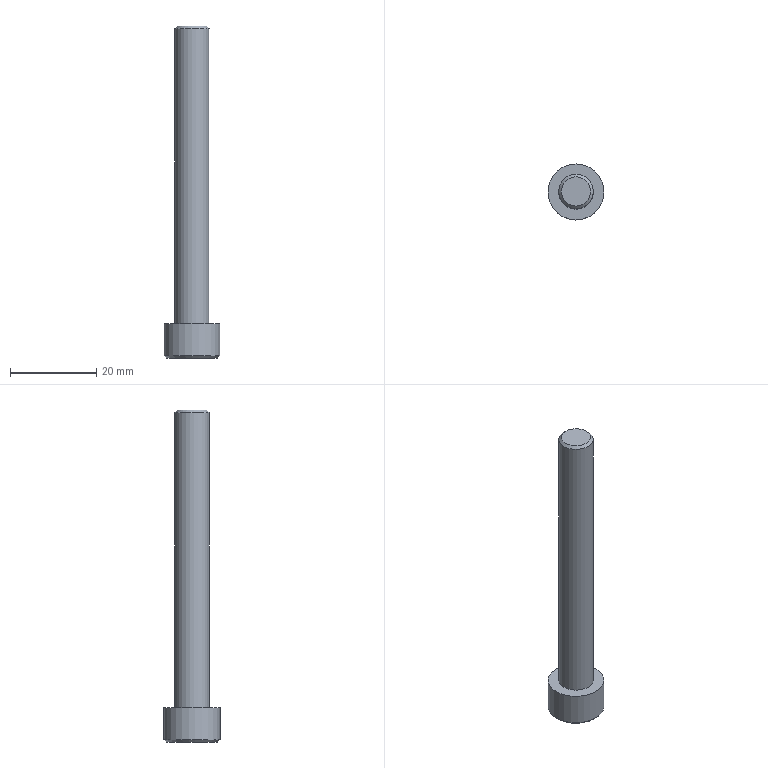Part | STEP file | gslz 2016.10.28-6_id210_x_t | 1 solid | 14 faces | box 13 x 13 x 77 mm | volume 4365 mm3 | plane 10 | cylinder 2 | cone 2 | commonest cylinder face diameters 8 x1 13 x1
STEP:
#1=CARTESIAN_POINT('',(-50.5,57.,67.992));
#2=VERTEX_POINT('',#1);
#3=CARTESIAN_POINT('',(-50.5,51.,67.992));
#4=DIRECTION('',(0.,0.,-1.));
#5=DIRECTION('',(0.,1.,0.));
#6=AXIS2_PLACEMENT_3D('',#3,#4,#5);
#7=CIRCLE('',#6,6.);
#8=EDGE_CURVE('',#2,#2,#7,.T.);
#9=ORIENTED_EDGE('',*,*,#8,.T.);
#10=EDGE_LOOP('',(#9));
#11=FACE_BOUND('',#10,.T.);
#12=CARTESIAN_POINT('',(-48.768,48.,67.992));
#13=VERTEX_POINT('',#12);
#14=CARTESIAN_POINT('',(-52.232,48.,67.992));
#15=VERTEX_POINT('',#14);
#16=CARTESIAN_POINT('',(-48.768,48.,67.992));
#17=DIRECTION('',(-1.,0.,0.));
#18=VECTOR('',#17,1.);
#19=LINE('',#16,#18);
#20=EDGE_CURVE('',#13,#15,#19,.T.);
#21=ORIENTED_EDGE('',*,*,#20,.F.);
#22=CARTESIAN_POINT('',(-47.036,51.,67.992));
#23=VERTEX_POINT('',#22);
#24=CARTESIAN_POINT('',(-47.036,51.,67.992));
#25=DIRECTION('',(-0.5,-0.866,0.));
#26=VECTOR('',#25,1.);
#27=LINE('',#24,#26);
#28=EDGE_CURVE('',#23,#13,#27,.T.);
#29=ORIENTED_EDGE('',*,*,#28,.F.);
#30=CARTESIAN_POINT('',(-48.768,54.,67.992));
#31=VERTEX_POINT('',#30);
#32=CARTESIAN_POINT('',(-48.768,54.,67.992));
#33=DIRECTION('',(0.5,-0.866,0.));
#34=VECTOR('',#33,1.);
#35=LINE('',#32,#34);
#36=EDGE_CURVE('',#31,#23,#35,.T.);
#37=ORIENTED_EDGE('',*,*,#36,.F.);
#38=CARTESIAN_POINT('',(-52.232,54.,67.992));
#39=VERTEX_POINT('',#38);
#40=CARTESIAN_POINT('',(-52.232,54.,67.992));
#41=DIRECTION('',(1.,0.,0.));
#42=VECTOR('',#41,1.);
#43=LINE('',#40,#42);
#44=EDGE_CURVE('',#39,#31,#43,.T.);
#45=ORIENTED_EDGE('',*,*,#44,.F.);
#46=CARTESIAN_POINT('',(-53.964,51.,67.992));
#47=VERTEX_POINT('',#46);
#48=CARTESIAN_POINT('',(-53.964,51.,67.992));
#49=DIRECTION('',(0.5,0.866,0.));
#50=VECTOR('',#49,1.);
#51=LINE('',#48,#50);
#52=EDGE_CURVE('',#47,#39,#51,.T.);
#53=ORIENTED_EDGE('',*,*,#52,.F.);
#54=CARTESIAN_POINT('',(-52.232,48.,67.992));
#55=DIRECTION('',(-0.5,0.866,0.));
#56=VECTOR('',#55,1.);
#57=LINE('',#54,#56);
#58=EDGE_CURVE('',#15,#47,#57,.T.);
#59=ORIENTED_EDGE('',*,*,#58,.F.);
#60=EDGE_LOOP('',(#21,#29,#37,#45,#53,#59));
#61=FACE_BOUND('',#60,.T.);
#62=CARTESIAN_POINT('',(-50.5,51.,67.992));
#63=DIRECTION('',(0.,0.,-1.));
#64=DIRECTION('',(0.,-1.,0.));
#65=AXIS2_PLACEMENT_3D('',#62,#63,#64);
#66=PLANE('',#65);
#67=ADVANCED_FACE('',(#11,#61),#66,.T.);
#68=CARTESIAN_POINT('',(-50.5,47.6,144.992));
#69=VERTEX_POINT('',#68);
#70=CARTESIAN_POINT('',(-50.5,51.,144.992));
#71=DIRECTION('',(0.,0.,1.));
#72=DIRECTION('',(0.,-1.,0.));
#73=AXIS2_PLACEMENT_3D('',#70,#71,#72);
#74=CIRCLE('',#73,3.4);
#75=EDGE_CURVE('',#69,#69,#74,.T.);
#76=ORIENTED_EDGE('',*,*,#75,.T.);
#77=EDGE_LOOP('',(#76));
#78=FACE_OUTER_BOUND('',#77,.T.);
#79=CARTESIAN_POINT('',(-50.5,51.,144.992));
#80=DIRECTION('',(0.,0.,1.));
#81=DIRECTION('',(0.,1.,0.));
#82=AXIS2_PLACEMENT_3D('',#79,#80,#81);
#83=PLANE('',#82);
#84=ADVANCED_FACE('',(#78),#83,.T.);
#85=CARTESIAN_POINT('',(-50.5,47.,144.392));
#86=VERTEX_POINT('',#85);
#87=CARTESIAN_POINT('',(-50.5,51.,144.392));
#88=DIRECTION('',(0.,0.,-1.));
#89=DIRECTION('',(0.,-1.,0.));
#90=AXIS2_PLACEMENT_3D('',#87,#88,#89);
#91=CIRCLE('',#90,4.);
#92=EDGE_CURVE('',#86,#86,#91,.T.);
#93=ORIENTED_EDGE('',*,*,#92,.T.);
#94=EDGE_LOOP('',(#93));
#95=FACE_BOUND('',#94,.T.);
#96=CARTESIAN_POINT('',(-50.5,47.,75.992));
#97=VERTEX_POINT('',#96);
#98=CARTESIAN_POINT('',(-50.5,51.,75.992));
#99=DIRECTION('',(0.,0.,1.));
#100=DIRECTION('',(0.,-1.,0.));
#101=AXIS2_PLACEMENT_3D('',#98,#99,#100);
#102=CIRCLE('',#101,4.);
#103=EDGE_CURVE('',#97,#97,#102,.T.);
#104=ORIENTED_EDGE('',*,*,#103,.T.);
#105=EDGE_LOOP('',(#104));
#106=FACE_BOUND('',#105,.T.);
#107=CARTESIAN_POINT('',(-50.5,51.,129.992));
#108=DIRECTION('',(0.,0.,1.));
#109=DIRECTION('',(1.,0.,0.));
#110=AXIS2_PLACEMENT_3D('',#107,#108,#109);
#111=CYLINDRICAL_SURFACE('',#110,4.);
#112=ADVANCED_FACE('',(#95,#106),#111,.T.);
#113=ORIENTED_EDGE('',*,*,#103,.F.);
#114=EDGE_LOOP('',(#113));
#115=FACE_BOUND('',#114,.T.);
#116=CARTESIAN_POINT('',(-50.5,44.5,75.992));
#117=VERTEX_POINT('',#116);
#118=CARTESIAN_POINT('',(-50.5,51.,75.992));
#119=DIRECTION('',(0.,0.,1.));
#120=DIRECTION('',(0.,-1.,0.));
#121=AXIS2_PLACEMENT_3D('',#118,#119,#120);
#122=CIRCLE('',#121,6.5);
#123=EDGE_CURVE('',#117,#117,#122,.T.);
#124=ORIENTED_EDGE('',*,*,#123,.T.);
#125=EDGE_LOOP('',(#124));
#126=FACE_BOUND('',#125,.T.);
#127=CARTESIAN_POINT('',(-50.5,51.,75.992));
#128=DIRECTION('',(0.,0.,1.));
#129=DIRECTION('',(0.,1.,0.));
#130=AXIS2_PLACEMENT_3D('',#127,#128,#129);
#131=PLANE('',#130);
#132=ADVANCED_FACE('',(#115,#126),#131,.T.);
#133=CARTESIAN_POINT('',(-50.5,57.5,68.492));
#134=VERTEX_POINT('',#133);
#135=CARTESIAN_POINT('',(-50.5,51.,68.492));
#136=DIRECTION('',(0.,0.,1.));
#137=DIRECTION('',(0.,1.,0.));
#138=AXIS2_PLACEMENT_3D('',#135,#136,#137);
#139=CIRCLE('',#138,6.5);
#140=EDGE_CURVE('',#134,#134,#139,.T.);
#141=ORIENTED_EDGE('',*,*,#140,.T.);
#142=EDGE_LOOP('',(#141));
#143=FACE_BOUND('',#142,.T.);
#144=ORIENTED_EDGE('',*,*,#123,.F.);
#145=EDGE_LOOP('',(#144));
#146=FACE_BOUND('',#145,.T.);
#147=CARTESIAN_POINT('',(-50.5,51.,64.992));
#148=DIRECTION('',(0.,0.,1.));
#149=DIRECTION('',(1.,0.,0.));
#150=AXIS2_PLACEMENT_3D('',#147,#148,#149);
#151=CYLINDRICAL_SURFACE('',#150,6.5);
#152=ADVANCED_FACE('',(#143,#146),#151,.T.);
#153=ORIENTED_EDGE('',*,*,#92,.F.);
#154=EDGE_LOOP('',(#153));
#155=FACE_BOUND('',#154,.T.);
#156=ORIENTED_EDGE('',*,*,#75,.F.);
#157=EDGE_LOOP('',(#156));
#158=FACE_BOUND('',#157,.T.);
#159=CARTESIAN_POINT('',(-50.5,51.,144.992));
#160=DIRECTION('',(0.,0.,-1.));
#161=DIRECTION('',(0.,1.,0.));
#162=AXIS2_PLACEMENT_3D('',#159,#160,#161);
#163=CONICAL_SURFACE('',#162,3.4,45.);
#164=ADVANCED_FACE('',(#155,#158),#163,.T.);
#165=ORIENTED_EDGE('',*,*,#20,.T.);
#166=CARTESIAN_POINT('',(-52.232,48.,72.992));
#167=VERTEX_POINT('',#166);
#168=CARTESIAN_POINT('',(-52.232,48.,72.992));
#169=DIRECTION('',(0.,0.,1.));
#170=VECTOR('',#169,1.);
#171=LINE('',#168,#170);
#172=EDGE_CURVE('',#15,#167,#171,.T.);
#173=ORIENTED_EDGE('',*,*,#172,.T.);
#174=CARTESIAN_POINT('',(-48.768,48.,72.992));
#175=VERTEX_POINT('',#174);
#176=CARTESIAN_POINT('',(-48.768,48.,72.992));
#177=DIRECTION('',(1.,0.,0.));
#178=VECTOR('',#177,1.);
#179=LINE('',#176,#178);
#180=EDGE_CURVE('',#167,#175,#179,.T.);
#181=ORIENTED_EDGE('',*,*,#180,.T.);
#182=CARTESIAN_POINT('',(-48.768,48.,72.992));
#183=DIRECTION('',(0.,0.,1.));
#184=VECTOR('',#183,1.);
#185=LINE('',#182,#184);
#186=EDGE_CURVE('',#13,#175,#185,.T.);
#187=ORIENTED_EDGE('',*,*,#186,.F.);
#188=EDGE_LOOP('',(#165,#173,#181,#187));
#189=FACE_OUTER_BOUND('',#188,.T.);
#190=CARTESIAN_POINT('',(-48.768,48.,72.992));
#191=DIRECTION('',(0.,-1.,0.));
#192=DIRECTION('',(0.,0.,-1.));
#193=AXIS2_PLACEMENT_3D('',#190,#191,#192);
#194=PLANE('',#193);
#195=ADVANCED_FACE('',(#189),#194,.F.);
#196=ORIENTED_EDGE('',*,*,#58,.T.);
#197=CARTESIAN_POINT('',(-53.964,51.,72.992));
#198=VERTEX_POINT('',#197);
#199=CARTESIAN_POINT('',(-53.964,51.,72.992));
#200=DIRECTION('',(0.,0.,1.));
#201=VECTOR('',#200,1.);
#202=LINE('',#199,#201);
#203=EDGE_CURVE('',#47,#198,#202,.T.);
#204=ORIENTED_EDGE('',*,*,#203,.T.);
#205=CARTESIAN_POINT('',(-52.232,48.,72.992));
#206=DIRECTION('',(0.5,-0.866,0.));
#207=VECTOR('',#206,1.);
#208=LINE('',#205,#207);
#209=EDGE_CURVE('',#198,#167,#208,.T.);
#210=ORIENTED_EDGE('',*,*,#209,.T.);
#211=ORIENTED_EDGE('',*,*,#172,.F.);
#212=EDGE_LOOP('',(#196,#204,#210,#211));
#213=FACE_OUTER_BOUND('',#212,.T.);
#214=CARTESIAN_POINT('',(-52.232,48.,72.992));
#215=DIRECTION('',(-0.866,-0.5,0.));
#216=DIRECTION('',(0.5,-0.866,0.));
#217=AXIS2_PLACEMENT_3D('',#214,#215,#216);
#218=PLANE('',#217);
#219=ADVANCED_FACE('',(#213),#218,.F.);
#220=ORIENTED_EDGE('',*,*,#52,.T.);
#221=CARTESIAN_POINT('',(-52.232,54.,72.992));
#222=VERTEX_POINT('',#221);
#223=CARTESIAN_POINT('',(-52.232,54.,72.992));
#224=DIRECTION('',(0.,0.,1.));
#225=VECTOR('',#224,1.);
#226=LINE('',#223,#225);
#227=EDGE_CURVE('',#39,#222,#226,.T.);
#228=ORIENTED_EDGE('',*,*,#227,.T.);
#229=CARTESIAN_POINT('',(-53.964,51.,72.992));
#230=DIRECTION('',(-0.5,-0.866,0.));
#231=VECTOR('',#230,1.);
#232=LINE('',#229,#231);
#233=EDGE_CURVE('',#222,#198,#232,.T.);
#234=ORIENTED_EDGE('',*,*,#233,.T.);
#235=ORIENTED_EDGE('',*,*,#203,.F.);
#236=EDGE_LOOP('',(#220,#228,#234,#235));
#237=FACE_OUTER_BOUND('',#236,.T.);
#238=CARTESIAN_POINT('',(-53.964,51.,72.992));
#239=DIRECTION('',(-0.866,0.5,0.));
#240=DIRECTION('',(-0.5,-0.866,0.));
#241=AXIS2_PLACEMENT_3D('',#238,#239,#240);
#242=PLANE('',#241);
#243=ADVANCED_FACE('',(#237),#242,.F.);
#244=ORIENTED_EDGE('',*,*,#44,.T.);
#245=CARTESIAN_POINT('',(-48.768,54.,72.992));
#246=VERTEX_POINT('',#245);
#247=CARTESIAN_POINT('',(-48.768,54.,72.992));
#248=DIRECTION('',(0.,0.,1.));
#249=VECTOR('',#248,1.);
#250=LINE('',#247,#249);
#251=EDGE_CURVE('',#31,#246,#250,.T.);
#252=ORIENTED_EDGE('',*,*,#251,.T.);
#253=CARTESIAN_POINT('',(-52.232,54.,72.992));
#254=DIRECTION('',(-1.,0.,0.));
#255=VECTOR('',#254,1.);
#256=LINE('',#253,#255);
#257=EDGE_CURVE('',#246,#222,#256,.T.);
#258=ORIENTED_EDGE('',*,*,#257,.T.);
#259=ORIENTED_EDGE('',*,*,#227,.F.);
#260=EDGE_LOOP('',(#244,#252,#258,#259));
#261=FACE_OUTER_BOUND('',#260,.T.);
#262=CARTESIAN_POINT('',(-52.232,54.,72.992));
#263=DIRECTION('',(0.,1.,0.));
#264=DIRECTION('',(0.,0.,-1.));
#265=AXIS2_PLACEMENT_3D('',#262,#263,#264);
#266=PLANE('',#265);
#267=ADVANCED_FACE('',(#261),#266,.F.);
#268=ORIENTED_EDGE('',*,*,#36,.T.);
#269=CARTESIAN_POINT('',(-47.036,51.,72.992));
#270=VERTEX_POINT('',#269);
#271=CARTESIAN_POINT('',(-47.036,51.,72.992));
#272=DIRECTION('',(0.,0.,1.));
#273=VECTOR('',#272,1.);
#274=LINE('',#271,#273);
#275=EDGE_CURVE('',#23,#270,#274,.T.);
#276=ORIENTED_EDGE('',*,*,#275,.T.);
#277=CARTESIAN_POINT('',(-48.768,54.,72.992));
#278=DIRECTION('',(-0.5,0.866,0.));
#279=VECTOR('',#278,1.);
#280=LINE('',#277,#279);
#281=EDGE_CURVE('',#270,#246,#280,.T.);
#282=ORIENTED_EDGE('',*,*,#281,.T.);
#283=ORIENTED_EDGE('',*,*,#251,.F.);
#284=EDGE_LOOP('',(#268,#276,#282,#283));
#285=FACE_OUTER_BOUND('',#284,.T.);
#286=CARTESIAN_POINT('',(-48.768,54.,72.992));
#287=DIRECTION('',(0.866,0.5,0.));
#288=DIRECTION('',(-0.5,0.866,0.));
#289=AXIS2_PLACEMENT_3D('',#286,#287,#288);
#290=PLANE('',#289);
#291=ADVANCED_FACE('',(#285),#290,.F.);
#292=ORIENTED_EDGE('',*,*,#28,.T.);
#293=ORIENTED_EDGE('',*,*,#186,.T.);
#294=CARTESIAN_POINT('',(-47.036,51.,72.992));
#295=DIRECTION('',(0.5,0.866,0.));
#296=VECTOR('',#295,1.);
#297=LINE('',#294,#296);
#298=EDGE_CURVE('',#175,#270,#297,.T.);
#299=ORIENTED_EDGE('',*,*,#298,.T.);
#300=ORIENTED_EDGE('',*,*,#275,.F.);
#301=EDGE_LOOP('',(#292,#293,#299,#300));
#302=FACE_OUTER_BOUND('',#301,.T.);
#303=CARTESIAN_POINT('',(-47.036,51.,72.992));
#304=DIRECTION('',(0.866,-0.5,0.));
#305=DIRECTION('',(0.5,0.866,0.));
#306=AXIS2_PLACEMENT_3D('',#303,#304,#305);
#307=PLANE('',#306);
#308=ADVANCED_FACE('',(#302),#307,.F.);
#309=ORIENTED_EDGE('',*,*,#180,.F.);
#310=ORIENTED_EDGE('',*,*,#209,.F.);
#311=ORIENTED_EDGE('',*,*,#233,.F.);
#312=ORIENTED_EDGE('',*,*,#257,.F.);
#313=ORIENTED_EDGE('',*,*,#281,.F.);
#314=ORIENTED_EDGE('',*,*,#298,.F.);
#315=EDGE_LOOP('',(#309,#310,#311,#312,#313,#314));
#316=FACE_OUTER_BOUND('',#315,.T.);
#317=CARTESIAN_POINT('',(-52.232,48.,72.992));
#318=DIRECTION('',(0.,0.,-1.));
#319=DIRECTION('',(0.,-1.,0.));
#320=AXIS2_PLACEMENT_3D('',#317,#318,#319);
#321=PLANE('',#320);
#322=ADVANCED_FACE('',(#316),#321,.T.);
#323=ORIENTED_EDGE('',*,*,#8,.F.);
#324=EDGE_LOOP('',(#323));
#325=FACE_BOUND('',#324,.T.);
#326=ORIENTED_EDGE('',*,*,#140,.F.);
#327=EDGE_LOOP('',(#326));
#328=FACE_BOUND('',#327,.T.);
#329=CARTESIAN_POINT('',(-50.5,51.,68.492));
#330=DIRECTION('',(0.,0.,1.));
#331=DIRECTION('',(1.,0.,0.));
#332=AXIS2_PLACEMENT_3D('',#329,#330,#331);
#333=CONICAL_SURFACE('',#332,6.5,45.);
#334=ADVANCED_FACE('',(#325,#328),#333,.T.);
#335=CLOSED_SHELL('',(#67,#84,#112,#132,#152,#164,#195,#219,#243,#267,#291,#308,#322,#334));
#336=MANIFOLD_SOLID_BREP('',#335);
#337=(LENGTH_UNIT()NAMED_UNIT(*)SI_UNIT(.MILLI.,.METRE.));
#338=UNCERTAINTY_MEASURE_WITH_UNIT(LENGTH_MEASURE(0.00002),#337,'','');
#339=(NAMED_UNIT(*)PLANE_ANGLE_UNIT()SI_UNIT($,.RADIAN.));
#340=PLANE_ANGLE_MEASURE_WITH_UNIT(PLANE_ANGLE_MEASURE(0.01745),#339);
#341=DIMENSIONAL_EXPONENTS(0.,0.,0.,0.,0.,0.,0.);
#342=(CONVERSION_BASED_UNIT('DEGREE',#340)NAMED_UNIT(#341)PLANE_ANGLE_UNIT());
#343=(NAMED_UNIT(*)SI_UNIT($,.STERADIAN.)SOLID_ANGLE_UNIT());
#344=(GEOMETRIC_REPRESENTATION_CONTEXT(3)GLOBAL_UNCERTAINTY_ASSIGNED_CONTEXT((#338))GLOBAL_UNIT_ASSIGNED_CONTEXT((#337,#342,#343))REPRESENTATION_CONTEXT('',''));
#345=ADVANCED_BREP_SHAPE_REPRESENTATION('',(#336),#344);